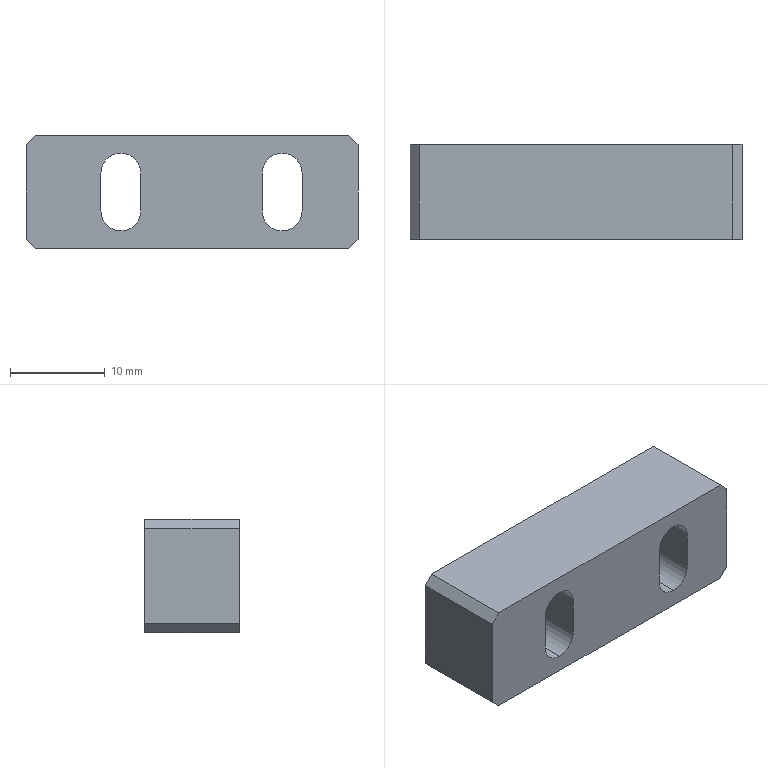Part | STEP file | PN_0005 | 1 solid | 20 faces | box 35 x 10 x 12 mm | volume 3567 mm3 | plane 14 | cylinder 6 | commonest cylinder face diameters 4.2 x6